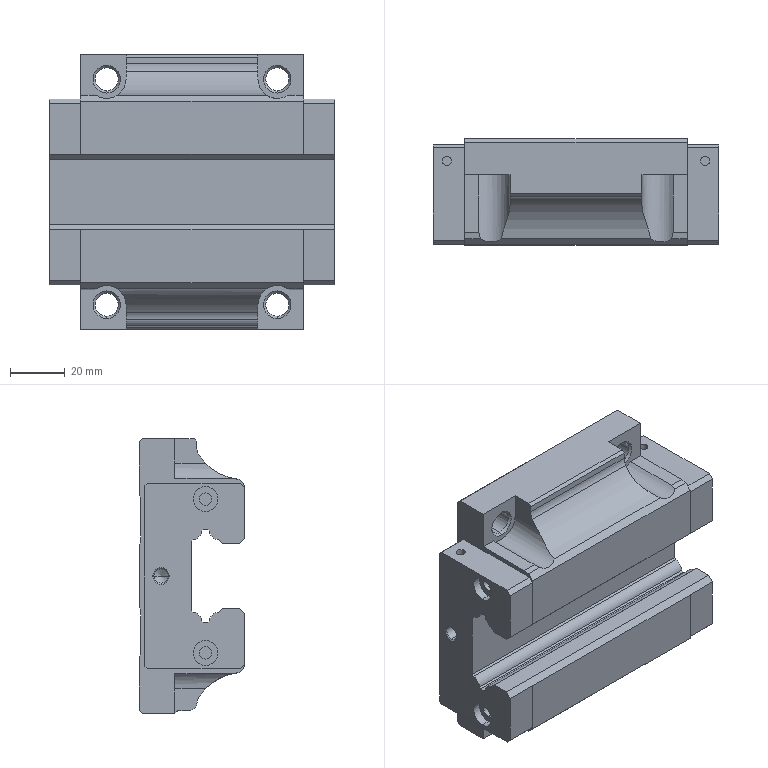Part | STEP file | _MSA35ESSFCN | 1 solid | 162 faces | box 104 x 38.5 x 100 mm | volume 261155 mm3 | plane 82 | cylinder 56 | cone 24 | commonest cylinder face diameters 3.3 x8 4.5 x8 8.376 x8 9 x8 14 x6 40 x6